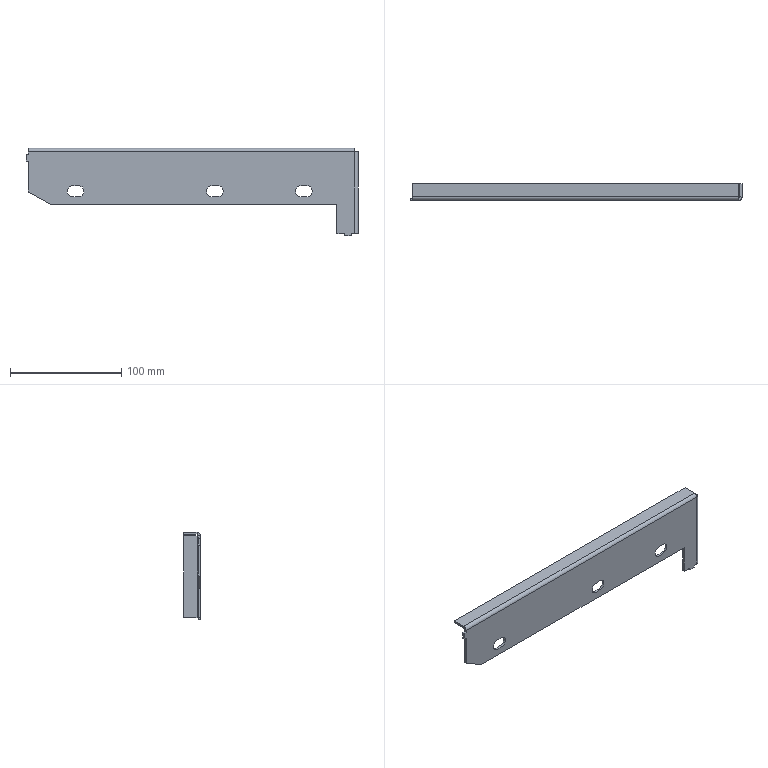Part | SolidWorks | features ICE 3, Cut 2, EdgeFlange 2, FlatPattern 1, SMBaseFlange 1, SheetMetal 1 | 1 solid | 45 faces | box 298 x 15 x 78.5 mm | volume 38712 mm3 | plane 35 | cylinder 10 | commonest cylinder face diameters 10 x6 2 x2 6 x2
STEP:
#1=CARTESIAN_POINT('',(-16.,0.,0.));
#2=VERTEX_POINT('',#1);
#3=CARTESIAN_POINT('',(-9.,0.,0.));
#4=VERTEX_POINT('',#3);
#5=CARTESIAN_POINT('',(-293.,0.,0.));
#6=DIRECTION('',(1.,0.,0.));
#7=VECTOR('',#6,1000.);
#8=LINE('',#5,#7);
#9=EDGE_CURVE('',#2,#4,#8,.T.);
#10=ORIENTED_EDGE('',*,*,#9,.T.);
#11=CARTESIAN_POINT('',(-9.,-2.,0.));
#12=VERTEX_POINT('',#11);
#13=CARTESIAN_POINT('',(-9.,0.,0.));
#14=DIRECTION('',(0.,1.,0.));
#15=VECTOR('',#14,1000.);
#16=LINE('',#13,#15);
#17=EDGE_CURVE('',#12,#4,#16,.T.);
#18=ORIENTED_EDGE('',*,*,#17,.F.);
#19=CARTESIAN_POINT('',(-16.,-2.,0.));
#20=VERTEX_POINT('',#19);
#21=CARTESIAN_POINT('',(-293.,-2.,0.));
#22=DIRECTION('',(1.,0.,0.));
#23=VECTOR('',#22,1000.);
#24=LINE('',#21,#23);
#25=EDGE_CURVE('',#20,#12,#24,.T.);
#26=ORIENTED_EDGE('',*,*,#25,.F.);
#27=CARTESIAN_POINT('',(-16.,0.,0.));
#28=DIRECTION('',(0.,-1.,0.));
#29=VECTOR('',#28,1000.);
#30=LINE('',#27,#29);
#31=EDGE_CURVE('',#2,#20,#30,.T.);
#32=ORIENTED_EDGE('',*,*,#31,.F.);
#33=EDGE_LOOP('',(#10,#18,#26,#32));
#34=FACE_OUTER_BOUND('',#33,.T.);
#35=CARTESIAN_POINT('',(0.,0.,0.));
#36=DIRECTION('',(0.,0.,-1.));
#37=DIRECTION('',(-1.,0.,0.));
#38=AXIS2_PLACEMENT_3D('',#35,#36,#37);
#39=PLANE('',#38);
#40=ADVANCED_FACE('',(#34),#39,.T.);
#41=CARTESIAN_POINT('',(-3.,-2.,0.));
#42=VERTEX_POINT('',#41);
#43=CARTESIAN_POINT('',(0.,-2.,0.));
#44=VERTEX_POINT('',#43);
#45=CARTESIAN_POINT('',(-293.,-2.,0.));
#46=DIRECTION('',(1.,0.,0.));
#47=VECTOR('',#46,1000.);
#48=LINE('',#45,#47);
#49=EDGE_CURVE('',#42,#44,#48,.T.);
#50=ORIENTED_EDGE('',*,*,#49,.F.);
#51=CARTESIAN_POINT('',(-3.,0.,0.));
#52=VERTEX_POINT('',#51);
#53=CARTESIAN_POINT('',(-3.,0.,0.));
#54=DIRECTION('',(0.,-1.,0.));
#55=VECTOR('',#54,1000.);
#56=LINE('',#53,#55);
#57=EDGE_CURVE('',#52,#42,#56,.T.);
#58=ORIENTED_EDGE('',*,*,#57,.F.);
#59=CARTESIAN_POINT('',(0.,0.,0.));
#60=VERTEX_POINT('',#59);
#61=CARTESIAN_POINT('',(-293.,0.,0.));
#62=DIRECTION('',(1.,0.,0.));
#63=VECTOR('',#62,1000.);
#64=LINE('',#61,#63);
#65=EDGE_CURVE('',#52,#60,#64,.T.);
#66=ORIENTED_EDGE('',*,*,#65,.T.);
#67=CARTESIAN_POINT('',(0.,0.,0.));
#68=DIRECTION('',(0.,-1.,0.));
#69=VECTOR('',#68,1000.);
#70=LINE('',#67,#69);
#71=EDGE_CURVE('',#60,#44,#70,.T.);
#72=ORIENTED_EDGE('',*,*,#71,.T.);
#73=EDGE_LOOP('',(#50,#58,#66,#72));
#74=FACE_OUTER_BOUND('',#73,.T.);
#75=CARTESIAN_POINT('',(0.,0.,0.));
#76=DIRECTION('',(0.,0.,-1.));
#77=DIRECTION('',(-1.,0.,0.));
#78=AXIS2_PLACEMENT_3D('',#75,#76,#77);
#79=PLANE('',#78);
#80=ADVANCED_FACE('',(#74),#79,.T.);
#81=CARTESIAN_POINT('',(-293.,0.,73.5));
#82=VERTEX_POINT('',#81);
#83=CARTESIAN_POINT('',(-293.,0.,71.));
#84=VERTEX_POINT('',#83);
#85=CARTESIAN_POINT('',(-293.,0.,73.5));
#86=DIRECTION('',(0.,0.,-1.));
#87=VECTOR('',#86,1000.);
#88=LINE('',#85,#87);
#89=EDGE_CURVE('',#82,#84,#88,.T.);
#90=ORIENTED_EDGE('',*,*,#89,.T.);
#91=CARTESIAN_POINT('',(-293.,-2.,71.));
#92=VERTEX_POINT('',#91);
#93=CARTESIAN_POINT('',(-293.,-2.,71.));
#94=DIRECTION('',(0.,1.,0.));
#95=VECTOR('',#94,1000.);
#96=LINE('',#93,#95);
#97=EDGE_CURVE('',#92,#84,#96,.T.);
#98=ORIENTED_EDGE('',*,*,#97,.F.);
#99=CARTESIAN_POINT('',(-293.,-2.,73.5));
#100=VERTEX_POINT('',#99);
#101=CARTESIAN_POINT('',(-293.,-2.,73.5));
#102=DIRECTION('',(0.,0.,-1.));
#103=VECTOR('',#102,1000.);
#104=LINE('',#101,#103);
#105=EDGE_CURVE('',#100,#92,#104,.T.);
#106=ORIENTED_EDGE('',*,*,#105,.F.);
#107=CARTESIAN_POINT('',(-293.,-2.,73.5));
#108=DIRECTION('',(0.,1.,0.));
#109=VECTOR('',#108,1000.);
#110=LINE('',#107,#109);
#111=EDGE_CURVE('',#100,#82,#110,.T.);
#112=ORIENTED_EDGE('',*,*,#111,.T.);
#113=EDGE_LOOP('',(#90,#98,#106,#112));
#114=FACE_OUTER_BOUND('',#113,.T.);
#115=CARTESIAN_POINT('',(-293.,-2.,73.5));
#116=DIRECTION('',(-1.,0.,0.));
#117=DIRECTION('',(0.,0.,1.));
#118=AXIS2_PLACEMENT_3D('',#115,#116,#117);
#119=PLANE('',#118);
#120=ADVANCED_FACE('',(#114),#119,.T.);
#121=CARTESIAN_POINT('',(-293.,-2.,65.));
#122=VERTEX_POINT('',#121);
#123=CARTESIAN_POINT('',(-293.,-2.,37.2));
#124=VERTEX_POINT('',#123);
#125=CARTESIAN_POINT('',(-293.,-2.,73.5));
#126=DIRECTION('',(0.,0.,-1.));
#127=VECTOR('',#126,1000.);
#128=LINE('',#125,#127);
#129=EDGE_CURVE('',#122,#124,#128,.T.);
#130=ORIENTED_EDGE('',*,*,#129,.F.);
#131=CARTESIAN_POINT('',(-293.,0.,65.));
#132=VERTEX_POINT('',#131);
#133=CARTESIAN_POINT('',(-293.,-2.,65.));
#134=DIRECTION('',(0.,-1.,0.));
#135=VECTOR('',#134,1000.);
#136=LINE('',#133,#135);
#137=EDGE_CURVE('',#132,#122,#136,.T.);
#138=ORIENTED_EDGE('',*,*,#137,.F.);
#139=CARTESIAN_POINT('',(-293.,0.,37.2));
#140=VERTEX_POINT('',#139);
#141=CARTESIAN_POINT('',(-293.,0.,73.5));
#142=DIRECTION('',(0.,0.,-1.));
#143=VECTOR('',#142,1000.);
#144=LINE('',#141,#143);
#145=EDGE_CURVE('',#132,#140,#144,.T.);
#146=ORIENTED_EDGE('',*,*,#145,.T.);
#147=CARTESIAN_POINT('',(-293.,8.,37.2));
#148=DIRECTION('',(0.,-1.,0.));
#149=VECTOR('',#148,1000.);
#150=LINE('',#147,#149);
#151=EDGE_CURVE('',#140,#124,#150,.T.);
#152=ORIENTED_EDGE('',*,*,#151,.T.);
#153=EDGE_LOOP('',(#130,#138,#146,#152));
#154=FACE_OUTER_BOUND('',#153,.T.);
#155=CARTESIAN_POINT('',(-293.,-2.,73.5));
#156=DIRECTION('',(-1.,0.,0.));
#157=DIRECTION('',(0.,0.,1.));
#158=AXIS2_PLACEMENT_3D('',#155,#156,#157);
#159=PLANE('',#158);
#160=ADVANCED_FACE('',(#154),#159,.T.);
#161=CARTESIAN_POINT('',(-253.,-2.,33.));
#162=VERTEX_POINT('',#161);
#163=CARTESIAN_POINT('',(-248.,-2.,33.));
#164=VERTEX_POINT('',#163);
#165=CARTESIAN_POINT('',(-253.,-2.,33.));
#166=DIRECTION('',(1.,0.,0.));
#167=VECTOR('',#166,1000.);
#168=LINE('',#165,#167);
#169=EDGE_CURVE('',#162,#164,#168,.T.);
#170=ORIENTED_EDGE('',*,*,#169,.F.);
#171=CARTESIAN_POINT('',(-253.,-2.,43.));
#172=VERTEX_POINT('',#171);
#173=CARTESIAN_POINT('',(-253.,-2.,38.));
#174=DIRECTION('',(0.,-1.,0.));
#175=DIRECTION('',(0.,0.,-1.));
#176=AXIS2_PLACEMENT_3D('',#173,#174,#175);
#177=CIRCLE('',#176,5.);
#178=EDGE_CURVE('',#172,#162,#177,.T.);
#179=ORIENTED_EDGE('',*,*,#178,.F.);
#180=CARTESIAN_POINT('',(-248.,-2.,43.));
#181=VERTEX_POINT('',#180);
#182=CARTESIAN_POINT('',(-253.,-2.,43.));
#183=DIRECTION('',(-1.,0.,0.));
#184=VECTOR('',#183,1000.);
#185=LINE('',#182,#184);
#186=EDGE_CURVE('',#181,#172,#185,.T.);
#187=ORIENTED_EDGE('',*,*,#186,.F.);
#188=CARTESIAN_POINT('',(-248.,-2.,38.));
#189=DIRECTION('',(0.,-1.,0.));
#190=DIRECTION('',(0.,0.,-1.));
#191=AXIS2_PLACEMENT_3D('',#188,#189,#190);
#192=CIRCLE('',#191,5.);
#193=EDGE_CURVE('',#164,#181,#192,.T.);
#194=ORIENTED_EDGE('',*,*,#193,.F.);
#195=EDGE_LOOP('',(#170,#179,#187,#194));
#196=FACE_BOUND('',#195,.T.);
#197=CARTESIAN_POINT('',(-128.,-2.,33.));
#198=VERTEX_POINT('',#197);
#199=CARTESIAN_POINT('',(-123.,-2.,33.));
#200=VERTEX_POINT('',#199);
#201=CARTESIAN_POINT('',(-128.,-2.,33.));
#202=DIRECTION('',(1.,0.,0.));
#203=VECTOR('',#202,1000.);
#204=LINE('',#201,#203);
#205=EDGE_CURVE('',#198,#200,#204,.T.);
#206=ORIENTED_EDGE('',*,*,#205,.F.);
#207=CARTESIAN_POINT('',(-128.,-2.,43.));
#208=VERTEX_POINT('',#207);
#209=CARTESIAN_POINT('',(-128.,-2.,38.));
#210=DIRECTION('',(0.,-1.,0.));
#211=DIRECTION('',(0.,0.,-1.));
#212=AXIS2_PLACEMENT_3D('',#209,#210,#211);
#213=CIRCLE('',#212,5.);
#214=EDGE_CURVE('',#208,#198,#213,.T.);
#215=ORIENTED_EDGE('',*,*,#214,.F.);
#216=CARTESIAN_POINT('',(-123.,-2.,43.));
#217=VERTEX_POINT('',#216);
#218=CARTESIAN_POINT('',(-128.,-2.,43.));
#219=DIRECTION('',(-1.,0.,0.));
#220=VECTOR('',#219,1000.);
#221=LINE('',#218,#220);
#222=EDGE_CURVE('',#217,#208,#221,.T.);
#223=ORIENTED_EDGE('',*,*,#222,.F.);
#224=CARTESIAN_POINT('',(-123.,-2.,38.));
#225=DIRECTION('',(0.,-1.,0.));
#226=DIRECTION('',(0.,0.,-1.));
#227=AXIS2_PLACEMENT_3D('',#224,#225,#226);
#228=CIRCLE('',#227,5.);
#229=EDGE_CURVE('',#200,#217,#228,.T.);
#230=ORIENTED_EDGE('',*,*,#229,.F.);
#231=EDGE_LOOP('',(#206,#215,#223,#230));
#232=FACE_BOUND('',#231,.T.);
#233=CARTESIAN_POINT('',(-48.,-2.,33.));
#234=VERTEX_POINT('',#233);
#235=CARTESIAN_POINT('',(-43.,-2.,33.));
#236=VERTEX_POINT('',#235);
#237=CARTESIAN_POINT('',(-48.,-2.,33.));
#238=DIRECTION('',(1.,0.,0.));
#239=VECTOR('',#238,1000.);
#240=LINE('',#237,#239);
#241=EDGE_CURVE('',#234,#236,#240,.T.);
#242=ORIENTED_EDGE('',*,*,#241,.F.);
#243=CARTESIAN_POINT('',(-48.,-2.,43.));
#244=VERTEX_POINT('',#243);
#245=CARTESIAN_POINT('',(-48.,-2.,38.));
#246=DIRECTION('',(0.,-1.,0.));
#247=DIRECTION('',(0.,0.,-1.));
#248=AXIS2_PLACEMENT_3D('',#245,#246,#247);
#249=CIRCLE('',#248,5.);
#250=EDGE_CURVE('',#244,#234,#249,.T.);
#251=ORIENTED_EDGE('',*,*,#250,.F.);
#252=CARTESIAN_POINT('',(-43.,-2.,43.));
#253=VERTEX_POINT('',#252);
#254=CARTESIAN_POINT('',(-48.,-2.,43.));
#255=DIRECTION('',(-1.,0.,0.));
#256=VECTOR('',#255,1000.);
#257=LINE('',#254,#256);
#258=EDGE_CURVE('',#253,#244,#257,.T.);
#259=ORIENTED_EDGE('',*,*,#258,.F.);
#260=CARTESIAN_POINT('',(-43.,-2.,38.));
#261=DIRECTION('',(0.,-1.,0.));
#262=DIRECTION('',(0.,0.,-1.));
#263=AXIS2_PLACEMENT_3D('',#260,#261,#262);
#264=CIRCLE('',#263,5.);
#265=EDGE_CURVE('',#236,#253,#264,.T.);
#266=ORIENTED_EDGE('',*,*,#265,.F.);
#267=EDGE_LOOP('',(#242,#251,#259,#266));
#268=FACE_BOUND('',#267,.T.);
#269=ORIENTED_EDGE('',*,*,#105,.T.);
#270=CARTESIAN_POINT('',(-295.,-2.,71.));
#271=VERTEX_POINT('',#270);
#272=CARTESIAN_POINT('',(-295.,-2.,71.));
#273=DIRECTION('',(1.,0.,0.));
#274=VECTOR('',#273,1000.);
#275=LINE('',#272,#274);
#276=EDGE_CURVE('',#271,#92,#275,.T.);
#277=ORIENTED_EDGE('',*,*,#276,.F.);
#278=CARTESIAN_POINT('',(-295.,-2.,65.));
#279=VERTEX_POINT('',#278);
#280=CARTESIAN_POINT('',(-295.,-2.,71.));
#281=DIRECTION('',(0.,0.,1.));
#282=VECTOR('',#281,1000.);
#283=LINE('',#280,#282);
#284=EDGE_CURVE('',#279,#271,#283,.T.);
#285=ORIENTED_EDGE('',*,*,#284,.F.);
#286=CARTESIAN_POINT('',(-295.,-2.,65.));
#287=DIRECTION('',(1.,0.,0.));
#288=VECTOR('',#287,1000.);
#289=LINE('',#286,#288);
#290=EDGE_CURVE('',#279,#122,#289,.T.);
#291=ORIENTED_EDGE('',*,*,#290,.T.);
#292=ORIENTED_EDGE('',*,*,#129,.T.);
#293=CARTESIAN_POINT('',(-273.,-2.,26.2));
#294=VERTEX_POINT('',#293);
#295=CARTESIAN_POINT('',(-293.,-2.,37.2));
#296=DIRECTION('',(-0.8762,0.,0.4819));
#297=VECTOR('',#296,1000.);
#298=LINE('',#295,#297);
#299=EDGE_CURVE('',#294,#124,#298,.T.);
#300=ORIENTED_EDGE('',*,*,#299,.F.);
#301=CARTESIAN_POINT('',(-16.,-2.,26.2));
#302=VERTEX_POINT('',#301);
#303=CARTESIAN_POINT('',(-293.,-2.,26.2));
#304=DIRECTION('',(-1.,0.,0.));
#305=VECTOR('',#304,1000.);
#306=LINE('',#303,#305);
#307=EDGE_CURVE('',#302,#294,#306,.T.);
#308=ORIENTED_EDGE('',*,*,#307,.F.);
#309=CARTESIAN_POINT('',(-16.,-2.,0.));
#310=DIRECTION('',(0.,0.,1.));
#311=VECTOR('',#310,1000.);
#312=LINE('',#309,#311);
#313=EDGE_CURVE('',#20,#302,#312,.T.);
#314=ORIENTED_EDGE('',*,*,#313,.F.);
#315=ORIENTED_EDGE('',*,*,#25,.T.);
#316=CARTESIAN_POINT('',(-9.,-2.,-2.));
#317=VERTEX_POINT('',#316);
#318=CARTESIAN_POINT('',(-9.,-2.,-2.));
#319=DIRECTION('',(0.,0.,1.));
#320=VECTOR('',#319,1000.);
#321=LINE('',#318,#320);
#322=EDGE_CURVE('',#317,#12,#321,.T.);
#323=ORIENTED_EDGE('',*,*,#322,.F.);
#324=CARTESIAN_POINT('',(-3.,-2.,-2.));
#325=VERTEX_POINT('',#324);
#326=CARTESIAN_POINT('',(-9.,-2.,-2.));
#327=DIRECTION('',(-1.,0.,0.));
#328=VECTOR('',#327,1000.);
#329=LINE('',#326,#328);
#330=EDGE_CURVE('',#325,#317,#329,.T.);
#331=ORIENTED_EDGE('',*,*,#330,.F.);
#332=CARTESIAN_POINT('',(-3.,-2.,-2.));
#333=DIRECTION('',(0.,0.,1.));
#334=VECTOR('',#333,1000.);
#335=LINE('',#332,#334);
#336=EDGE_CURVE('',#325,#42,#335,.T.);
#337=ORIENTED_EDGE('',*,*,#336,.T.);
#338=ORIENTED_EDGE('',*,*,#49,.T.);
#339=CARTESIAN_POINT('',(0.,-2.,73.5));
#340=VERTEX_POINT('',#339);
#341=CARTESIAN_POINT('',(0.,-2.,73.5));
#342=DIRECTION('',(0.,0.,-1.));
#343=VECTOR('',#342,1000.);
#344=LINE('',#341,#343);
#345=EDGE_CURVE('',#340,#44,#344,.T.);
#346=ORIENTED_EDGE('',*,*,#345,.F.);
#347=CARTESIAN_POINT('',(-293.,-2.,73.5));
#348=DIRECTION('',(1.,0.,0.));
#349=VECTOR('',#348,1000.);
#350=LINE('',#347,#349);
#351=EDGE_CURVE('',#100,#340,#350,.T.);
#352=ORIENTED_EDGE('',*,*,#351,.F.);
#353=EDGE_LOOP('',(#269,#277,#285,#291,#292,#300,#308,#314,#315,#323,#331,#337,#338,#346,#352));
#354=FACE_OUTER_BOUND('',#353,.T.);
#355=CARTESIAN_POINT('',(-293.,-2.,73.5));
#356=DIRECTION('',(0.,1.,0.));
#357=DIRECTION('',(0.,0.,1.));
#358=AXIS2_PLACEMENT_3D('',#355,#356,#357);
#359=PLANE('',#358);
#360=ADVANCED_FACE('',(#196,#232,#268,#354),#359,.F.);
#361=CARTESIAN_POINT('',(-273.,0.,26.2));
#362=VERTEX_POINT('',#361);
#363=CARTESIAN_POINT('',(-308.328,0.,45.631));
#364=DIRECTION('',(0.8762,0.,-0.4819));
#365=VECTOR('',#364,1000.);
#366=LINE('',#363,#365);
#367=EDGE_CURVE('',#140,#362,#366,.T.);
#368=ORIENTED_EDGE('',*,*,#367,.F.);
#369=ORIENTED_EDGE('',*,*,#145,.F.);
#370=CARTESIAN_POINT('',(-295.,0.,65.));
#371=VERTEX_POINT('',#370);
#372=CARTESIAN_POINT('',(-295.,0.,65.));
#373=DIRECTION('',(1.,0.,0.));
#374=VECTOR('',#373,1000.);
#375=LINE('',#372,#374);
#376=EDGE_CURVE('',#371,#132,#375,.T.);
#377=ORIENTED_EDGE('',*,*,#376,.F.);
#378=CARTESIAN_POINT('',(-295.,0.,71.));
#379=VERTEX_POINT('',#378);
#380=CARTESIAN_POINT('',(-295.,0.,71.));
#381=DIRECTION('',(0.,0.,-1.));
#382=VECTOR('',#381,1000.);
#383=LINE('',#380,#382);
#384=EDGE_CURVE('',#379,#371,#383,.T.);
#385=ORIENTED_EDGE('',*,*,#384,.F.);
#386=CARTESIAN_POINT('',(-295.,0.,71.));
#387=DIRECTION('',(1.,0.,0.));
#388=VECTOR('',#387,1000.);
#389=LINE('',#386,#388);
#390=EDGE_CURVE('',#379,#84,#389,.T.);
#391=ORIENTED_EDGE('',*,*,#390,.T.);
#392=ORIENTED_EDGE('',*,*,#89,.F.);
#393=CARTESIAN_POINT('',(0.,0.,73.5));
#394=VERTEX_POINT('',#393);
#395=CARTESIAN_POINT('',(-293.,0.,73.5));
#396=DIRECTION('',(1.,0.,0.));
#397=VECTOR('',#396,1000.);
#398=LINE('',#395,#397);
#399=EDGE_CURVE('',#82,#394,#398,.T.);
#400=ORIENTED_EDGE('',*,*,#399,.T.);
#401=CARTESIAN_POINT('',(0.,0.,73.5));
#402=DIRECTION('',(0.,0.,-1.));
#403=VECTOR('',#402,1000.);
#404=LINE('',#401,#403);
#405=EDGE_CURVE('',#394,#60,#404,.T.);
#406=ORIENTED_EDGE('',*,*,#405,.T.);
#407=ORIENTED_EDGE('',*,*,#65,.F.);
#408=CARTESIAN_POINT('',(-3.,0.,-2.));
#409=VERTEX_POINT('',#408);
#410=CARTESIAN_POINT('',(-3.,0.,-2.));
#411=DIRECTION('',(0.,0.,1.));
#412=VECTOR('',#411,1000.);
#413=LINE('',#410,#412);
#414=EDGE_CURVE('',#409,#52,#413,.T.);
#415=ORIENTED_EDGE('',*,*,#414,.F.);
#416=CARTESIAN_POINT('',(-9.,0.,-2.));
#417=VERTEX_POINT('',#416);
#418=CARTESIAN_POINT('',(-9.,0.,-2.));
#419=DIRECTION('',(1.,0.,0.));
#420=VECTOR('',#419,1000.);
#421=LINE('',#418,#420);
#422=EDGE_CURVE('',#417,#409,#421,.T.);
#423=ORIENTED_EDGE('',*,*,#422,.F.);
#424=CARTESIAN_POINT('',(-9.,0.,-2.));
#425=DIRECTION('',(0.,0.,1.));
#426=VECTOR('',#425,1000.);
#427=LINE('',#424,#426);
#428=EDGE_CURVE('',#417,#4,#427,.T.);
#429=ORIENTED_EDGE('',*,*,#428,.T.);
#430=ORIENTED_EDGE('',*,*,#9,.F.);
#431=CARTESIAN_POINT('',(-16.,0.,26.2));
#432=VERTEX_POINT('',#431);
#433=CARTESIAN_POINT('',(-16.,0.,73.5));
#434=DIRECTION('',(0.,0.,-1.));
#435=VECTOR('',#434,1000.);
#436=LINE('',#433,#435);
#437=EDGE_CURVE('',#432,#2,#436,.T.);
#438=ORIENTED_EDGE('',*,*,#437,.F.);
#439=CARTESIAN_POINT('',(-293.,0.,26.2));
#440=DIRECTION('',(1.,0.,0.));
#441=VECTOR('',#440,1000.);
#442=LINE('',#439,#441);
#443=EDGE_CURVE('',#362,#432,#442,.T.);
#444=ORIENTED_EDGE('',*,*,#443,.F.);
#445=EDGE_LOOP('',(#368,#369,#377,#385,#391,#392,#400,#406,#407,#415,#423,#429,#430,#438,#444));
#446=FACE_OUTER_BOUND('',#445,.T.);
#447=CARTESIAN_POINT('',(-253.,0.,33.));
#448=VERTEX_POINT('',#447);
#449=CARTESIAN_POINT('',(-253.,0.,43.));
#450=VERTEX_POINT('',#449);
#451=CARTESIAN_POINT('',(-253.,0.,38.));
#452=DIRECTION('',(0.,1.,0.));
#453=DIRECTION('',(0.,0.,1.));
#454=AXIS2_PLACEMENT_3D('',#451,#452,#453);
#455=CIRCLE('',#454,5.);
#456=EDGE_CURVE('',#448,#450,#455,.T.);
#457=ORIENTED_EDGE('',*,*,#456,.F.);
#458=CARTESIAN_POINT('',(-248.,0.,33.));
#459=VERTEX_POINT('',#458);
#460=CARTESIAN_POINT('',(-293.,0.,33.));
#461=DIRECTION('',(-1.,0.,0.));
#462=VECTOR('',#461,1000.);
#463=LINE('',#460,#462);
#464=EDGE_CURVE('',#459,#448,#463,.T.);
#465=ORIENTED_EDGE('',*,*,#464,.F.);
#466=CARTESIAN_POINT('',(-248.,0.,43.));
#467=VERTEX_POINT('',#466);
#468=CARTESIAN_POINT('',(-248.,0.,38.));
#469=DIRECTION('',(0.,1.,0.));
#470=DIRECTION('',(0.,0.,1.));
#471=AXIS2_PLACEMENT_3D('',#468,#469,#470);
#472=CIRCLE('',#471,5.);
#473=EDGE_CURVE('',#467,#459,#472,.T.);
#474=ORIENTED_EDGE('',*,*,#473,.F.);
#475=CARTESIAN_POINT('',(-293.,0.,43.));
#476=DIRECTION('',(1.,0.,0.));
#477=VECTOR('',#476,1000.);
#478=LINE('',#475,#477);
#479=EDGE_CURVE('',#450,#467,#478,.T.);
#480=ORIENTED_EDGE('',*,*,#479,.F.);
#481=EDGE_LOOP('',(#457,#465,#474,#480));
#482=FACE_BOUND('',#481,.T.);
#483=CARTESIAN_POINT('',(-128.,0.,33.));
#484=VERTEX_POINT('',#483);
#485=CARTESIAN_POINT('',(-128.,0.,43.));
#486=VERTEX_POINT('',#485);
#487=CARTESIAN_POINT('',(-128.,0.,38.));
#488=DIRECTION('',(0.,1.,0.));
#489=DIRECTION('',(0.,0.,1.));
#490=AXIS2_PLACEMENT_3D('',#487,#488,#489);
#491=CIRCLE('',#490,5.);
#492=EDGE_CURVE('',#484,#486,#491,.T.);
#493=ORIENTED_EDGE('',*,*,#492,.F.);
#494=CARTESIAN_POINT('',(-123.,0.,33.));
#495=VERTEX_POINT('',#494);
#496=CARTESIAN_POINT('',(-293.,0.,33.));
#497=DIRECTION('',(-1.,0.,0.));
#498=VECTOR('',#497,1000.);
#499=LINE('',#496,#498);
#500=EDGE_CURVE('',#495,#484,#499,.T.);
#501=ORIENTED_EDGE('',*,*,#500,.F.);
#502=CARTESIAN_POINT('',(-123.,0.,43.));
#503=VERTEX_POINT('',#502);
#504=CARTESIAN_POINT('',(-123.,0.,38.));
#505=DIRECTION('',(0.,1.,0.));
#506=DIRECTION('',(0.,0.,1.));
#507=AXIS2_PLACEMENT_3D('',#504,#505,#506);
#508=CIRCLE('',#507,5.);
#509=EDGE_CURVE('',#503,#495,#508,.T.);
#510=ORIENTED_EDGE('',*,*,#509,.F.);
#511=CARTESIAN_POINT('',(-293.,0.,43.));
#512=DIRECTION('',(1.,0.,0.));
#513=VECTOR('',#512,1000.);
#514=LINE('',#511,#513);
#515=EDGE_CURVE('',#486,#503,#514,.T.);
#516=ORIENTED_EDGE('',*,*,#515,.F.);
#517=EDGE_LOOP('',(#493,#501,#510,#516));
#518=FACE_BOUND('',#517,.T.);
#519=CARTESIAN_POINT('',(-48.,0.,33.));
#520=VERTEX_POINT('',#519);
#521=CARTESIAN_POINT('',(-48.,0.,43.));
#522=VERTEX_POINT('',#521);
#523=CARTESIAN_POINT('',(-48.,0.,38.));
#524=DIRECTION('',(0.,1.,0.));
#525=DIRECTION('',(0.,0.,1.));
#526=AXIS2_PLACEMENT_3D('',#523,#524,#525);
#527=CIRCLE('',#526,5.);
#528=EDGE_CURVE('',#520,#522,#527,.T.);
#529=ORIENTED_EDGE('',*,*,#528,.F.);
#530=CARTESIAN_POINT('',(-43.,0.,33.));
#531=VERTEX_POINT('',#530);
#532=CARTESIAN_POINT('',(-293.,0.,33.));
#533=DIRECTION('',(-1.,0.,0.));
#534=VECTOR('',#533,1000.);
#535=LINE('',#532,#534);
#536=EDGE_CURVE('',#531,#520,#535,.T.);
#537=ORIENTED_EDGE('',*,*,#536,.F.);
#538=CARTESIAN_POINT('',(-43.,0.,43.));
#539=VERTEX_POINT('',#538);
#540=CARTESIAN_POINT('',(-43.,0.,38.));
#541=DIRECTION('',(0.,1.,0.));
#542=DIRECTION('',(0.,0.,1.));
#543=AXIS2_PLACEMENT_3D('',#540,#541,#542);
#544=CIRCLE('',#543,5.);
#545=EDGE_CURVE('',#539,#531,#544,.T.);
#546=ORIENTED_EDGE('',*,*,#545,.F.);
#547=CARTESIAN_POINT('',(-293.,0.,43.));
#548=DIRECTION('',(1.,0.,0.));
#549=VECTOR('',#548,1000.);
#550=LINE('',#547,#549);
#551=EDGE_CURVE('',#522,#539,#550,.T.);
#552=ORIENTED_EDGE('',*,*,#551,.F.);
#553=EDGE_LOOP('',(#529,#537,#546,#552));
#554=FACE_BOUND('',#553,.T.);
#555=CARTESIAN_POINT('',(-293.,0.,73.5));
#556=DIRECTION('',(0.,1.,0.));
#557=DIRECTION('',(0.,0.,1.));
#558=AXIS2_PLACEMENT_3D('',#555,#556,#557);
#559=PLANE('',#558);
#560=ADVANCED_FACE('',(#446,#482,#518,#554),#559,.T.);
#561=CARTESIAN_POINT('',(-293.,1.,74.5));
#562=VERTEX_POINT('',#561);
#563=CARTESIAN_POINT('',(-293.,1.,76.5));
#564=VERTEX_POINT('',#563);
#565=CARTESIAN_POINT('',(-293.,1.,76.5));
#566=DIRECTION('',(0.,0.,1.));
#567=VECTOR('',#566,1000.);
#568=LINE('',#565,#567);
#569=EDGE_CURVE('',#562,#564,#568,.T.);
#570=ORIENTED_EDGE('',*,*,#569,.F.);
#571=CARTESIAN_POINT('',(-293.,1.,73.5));
#572=DIRECTION('',(-1.,0.,0.));
#573=DIRECTION('',(0.,0.,-1.));
#574=AXIS2_PLACEMENT_3D('',#571,#572,#573);
#575=CIRCLE('',#574,1.);
#576=EDGE_CURVE('',#82,#562,#575,.T.);
#577=ORIENTED_EDGE('',*,*,#576,.F.);
#578=ORIENTED_EDGE('',*,*,#111,.F.);
#579=CARTESIAN_POINT('',(-293.,1.,73.5));
#580=DIRECTION('',(-1.,0.,0.));
#581=DIRECTION('',(0.,0.,-1.));
#582=AXIS2_PLACEMENT_3D('',#579,#580,#581);
#583=CIRCLE('',#582,3.);
#584=EDGE_CURVE('',#100,#564,#583,.T.);
#585=ORIENTED_EDGE('',*,*,#584,.T.);
#586=EDGE_LOOP('',(#570,#577,#578,#585));
#587=FACE_OUTER_BOUND('',#586,.T.);
#588=CARTESIAN_POINT('',(-293.,1.,73.5));
#589=DIRECTION('',(-1.,0.,0.));
#590=DIRECTION('',(0.,0.,1.));
#591=AXIS2_PLACEMENT_3D('',#588,#589,#590);
#592=PLANE('',#591);
#593=ADVANCED_FACE('',(#587),#592,.T.);
#594=CARTESIAN_POINT('',(0.,1.,74.5));
#595=VERTEX_POINT('',#594);
#596=CARTESIAN_POINT('',(0.,1.,73.5));
#597=DIRECTION('',(1.,0.,0.));
#598=DIRECTION('',(0.,0.,-1.));
#599=AXIS2_PLACEMENT_3D('',#596,#597,#598);
#600=CIRCLE('',#599,1.);
#601=EDGE_CURVE('',#595,#394,#600,.T.);
#602=ORIENTED_EDGE('',*,*,#601,.F.);
#603=CARTESIAN_POINT('',(0.,1.,76.5));
#604=VERTEX_POINT('',#603);
#605=CARTESIAN_POINT('',(0.,1.,74.5));
#606=DIRECTION('',(0.,0.,1.));
#607=VECTOR('',#606,1000.);
#608=LINE('',#605,#607);
#609=EDGE_CURVE('',#595,#604,#608,.T.);
#610=ORIENTED_EDGE('',*,*,#609,.T.);
#611=CARTESIAN_POINT('',(0.,1.,73.5));
#612=DIRECTION('',(1.,0.,0.));
#613=DIRECTION('',(0.,0.,-1.));
#614=AXIS2_PLACEMENT_3D('',#611,#612,#613);
#615=CIRCLE('',#614,3.);
#616=EDGE_CURVE('',#604,#340,#615,.T.);
#617=ORIENTED_EDGE('',*,*,#616,.T.);
#618=CARTESIAN_POINT('',(0.,0.,73.5));
#619=DIRECTION('',(0.,-1.,0.));
#620=VECTOR('',#619,1000.);
#621=LINE('',#618,#620);
#622=EDGE_CURVE('',#394,#340,#621,.T.);
#623=ORIENTED_EDGE('',*,*,#622,.F.);
#624=EDGE_LOOP('',(#602,#610,#617,#623));
#625=FACE_OUTER_BOUND('',#624,.T.);
#626=CARTESIAN_POINT('',(0.,1.,73.5));
#627=DIRECTION('',(-1.,0.,0.));
#628=DIRECTION('',(0.,0.,1.));
#629=AXIS2_PLACEMENT_3D('',#626,#627,#628);
#630=PLANE('',#629);
#631=ADVANCED_FACE('',(#625),#630,.F.);
#632=ORIENTED_EDGE('',*,*,#351,.T.);
#633=ORIENTED_EDGE('',*,*,#616,.F.);
#634=CARTESIAN_POINT('',(-293.,1.,76.5));
#635=DIRECTION('',(-1.,0.,0.));
#636=VECTOR('',#635,1000.);
#637=LINE('',#634,#636);
#638=EDGE_CURVE('',#604,#564,#637,.T.);
#639=ORIENTED_EDGE('',*,*,#638,.T.);
#640=ORIENTED_EDGE('',*,*,#584,.F.);
#641=EDGE_LOOP('',(#632,#633,#639,#640));
#642=FACE_OUTER_BOUND('',#641,.T.);
#643=CARTESIAN_POINT('',(0.,1.,73.5));
#644=DIRECTION('',(1.,0.,0.));
#645=DIRECTION('',(0.,0.,1.));
#646=AXIS2_PLACEMENT_3D('',#643,#644,#645);
#647=CYLINDRICAL_SURFACE('',#646,3.);
#648=ADVANCED_FACE('',(#642),#647,.T.);
#649=ORIENTED_EDGE('',*,*,#399,.F.);
#650=ORIENTED_EDGE('',*,*,#576,.T.);
#651=CARTESIAN_POINT('',(-293.,1.,74.5));
#652=DIRECTION('',(1.,0.,0.));
#653=VECTOR('',#652,1000.);
#654=LINE('',#651,#653);
#655=EDGE_CURVE('',#562,#595,#654,.T.);
#656=ORIENTED_EDGE('',*,*,#655,.T.);
#657=ORIENTED_EDGE('',*,*,#601,.T.);
#658=EDGE_LOOP('',(#649,#650,#656,#657));
#659=FACE_OUTER_BOUND('',#658,.T.);
#660=CARTESIAN_POINT('',(0.,1.,73.5));
#661=DIRECTION('',(1.,0.,0.));
#662=DIRECTION('',(0.,0.,1.));
#663=AXIS2_PLACEMENT_3D('',#660,#661,#662);
#664=CYLINDRICAL_SURFACE('',#663,1.);
#665=ADVANCED_FACE('',(#659),#664,.F.);
#666=ORIENTED_EDGE('',*,*,#569,.T.);
#667=CARTESIAN_POINT('',(-293.,13.,76.5));
#668=VERTEX_POINT('',#667);
#669=CARTESIAN_POINT('',(-293.,0.,76.5));
#670=DIRECTION('',(0.,-1.,0.));
#671=VECTOR('',#670,1000.);
#672=LINE('',#669,#671);
#673=EDGE_CURVE('',#668,#564,#672,.T.);
#674=ORIENTED_EDGE('',*,*,#673,.F.);
#675=CARTESIAN_POINT('',(-293.,13.,74.5));
#676=VERTEX_POINT('',#675);
#677=CARTESIAN_POINT('',(-293.,13.,76.5));
#678=DIRECTION('',(0.,0.,-1.));
#679=VECTOR('',#678,1000.);
#680=LINE('',#677,#679);
#681=EDGE_CURVE('',#668,#676,#680,.T.);
#682=ORIENTED_EDGE('',*,*,#681,.T.);
#683=CARTESIAN_POINT('',(-293.,0.,74.5));
#684=DIRECTION('',(0.,-1.,0.));
#685=VECTOR('',#684,1000.);
#686=LINE('',#683,#685);
#687=EDGE_CURVE('',#676,#562,#686,.T.);
#688=ORIENTED_EDGE('',*,*,#687,.T.);
#689=EDGE_LOOP('',(#666,#674,#682,#688));
#690=FACE_OUTER_BOUND('',#689,.T.);
#691=CARTESIAN_POINT('',(-293.,0.,76.5));
#692=DIRECTION('',(1.,0.,0.));
#693=DIRECTION('',(0.,0.,-1.));
#694=AXIS2_PLACEMENT_3D('',#691,#692,#693);
#695=PLANE('',#694);
#696=ADVANCED_FACE('',(#690),#695,.F.);
#697=ORIENTED_EDGE('',*,*,#609,.F.);
#698=CARTESIAN_POINT('',(0.,13.,74.5));
#699=VERTEX_POINT('',#698);
#700=CARTESIAN_POINT('',(0.,13.,74.5));
#701=DIRECTION('',(0.,1.,0.));
#702=VECTOR('',#701,1000.);
#703=LINE('',#700,#702);
#704=EDGE_CURVE('',#595,#699,#703,.T.);
#705=ORIENTED_EDGE('',*,*,#704,.T.);
#706=CARTESIAN_POINT('',(0.,13.,76.5));
#707=VERTEX_POINT('',#706);
#708=CARTESIAN_POINT('',(0.,13.,76.5));
#709=DIRECTION('',(0.,0.,-1.));
#710=VECTOR('',#709,1000.);
#711=LINE('',#708,#710);
#712=EDGE_CURVE('',#707,#699,#711,.T.);
#713=ORIENTED_EDGE('',*,*,#712,.F.);
#714=CARTESIAN_POINT('',(0.,0.,76.5));
#715=DIRECTION('',(0.,1.,0.));
#716=VECTOR('',#715,1000.);
#717=LINE('',#714,#716);
#718=EDGE_CURVE('',#604,#707,#717,.T.);
#719=ORIENTED_EDGE('',*,*,#718,.F.);
#720=EDGE_LOOP('',(#697,#705,#713,#719));
#721=FACE_OUTER_BOUND('',#720,.T.);
#722=CARTESIAN_POINT('',(0.,13.,76.5));
#723=DIRECTION('',(-1.,0.,0.));
#724=DIRECTION('',(0.,-1.,0.));
#725=AXIS2_PLACEMENT_3D('',#722,#723,#724);
#726=PLANE('',#725);
#727=ADVANCED_FACE('',(#721),#726,.F.);
#728=ORIENTED_EDGE('',*,*,#638,.F.);
#729=ORIENTED_EDGE('',*,*,#718,.T.);
#730=CARTESIAN_POINT('',(0.,13.,76.5));
#731=DIRECTION('',(-1.,0.,0.));
#732=VECTOR('',#731,1000.);
#733=LINE('',#730,#732);
#734=EDGE_CURVE('',#707,#668,#733,.T.);
#735=ORIENTED_EDGE('',*,*,#734,.T.);
#736=ORIENTED_EDGE('',*,*,#673,.T.);
#737=EDGE_LOOP('',(#728,#729,#735,#736));
#738=FACE_OUTER_BOUND('',#737,.T.);
#739=CARTESIAN_POINT('',(0.,0.,76.5));
#740=DIRECTION('',(0.,0.,-1.));
#741=DIRECTION('',(-1.,0.,0.));
#742=AXIS2_PLACEMENT_3D('',#739,#740,#741);
#743=PLANE('',#742);
#744=ADVANCED_FACE('',(#738),#743,.F.);
#745=ORIENTED_EDGE('',*,*,#704,.F.);
#746=ORIENTED_EDGE('',*,*,#655,.F.);
#747=ORIENTED_EDGE('',*,*,#687,.F.);
#748=CARTESIAN_POINT('',(-293.,13.,74.5));
#749=DIRECTION('',(-1.,0.,0.));
#750=VECTOR('',#749,1000.);
#751=LINE('',#748,#750);
#752=EDGE_CURVE('',#699,#676,#751,.T.);
#753=ORIENTED_EDGE('',*,*,#752,.F.);
#754=EDGE_LOOP('',(#745,#746,#747,#753));
#755=FACE_OUTER_BOUND('',#754,.T.);
#756=CARTESIAN_POINT('',(0.,0.,74.5));
#757=DIRECTION('',(0.,0.,-1.));
#758=DIRECTION('',(-1.,0.,0.));
#759=AXIS2_PLACEMENT_3D('',#756,#757,#758);
#760=PLANE('',#759);
#761=ADVANCED_FACE('',(#755),#760,.T.);
#762=ORIENTED_EDGE('',*,*,#752,.T.);
#763=ORIENTED_EDGE('',*,*,#681,.F.);
#764=ORIENTED_EDGE('',*,*,#734,.F.);
#765=ORIENTED_EDGE('',*,*,#712,.T.);
#766=EDGE_LOOP('',(#762,#763,#764,#765));
#767=FACE_OUTER_BOUND('',#766,.T.);
#768=CARTESIAN_POINT('',(-293.,13.,76.5));
#769=DIRECTION('',(0.,-1.,0.));
#770=DIRECTION('',(0.,0.,-1.));
#771=AXIS2_PLACEMENT_3D('',#768,#769,#770);
#772=PLANE('',#771);
#773=ADVANCED_FACE('',(#767),#772,.F.);
#774=CARTESIAN_POINT('',(1.,1.,73.5));
#775=VERTEX_POINT('',#774);
#776=CARTESIAN_POINT('',(3.,1.,73.5));
#777=VERTEX_POINT('',#776);
#778=CARTESIAN_POINT('',(3.,1.,73.5));
#779=DIRECTION('',(1.,0.,0.));
#780=VECTOR('',#779,1000.);
#781=LINE('',#778,#780);
#782=EDGE_CURVE('',#775,#777,#781,.T.);
#783=ORIENTED_EDGE('',*,*,#782,.F.);
#784=CARTESIAN_POINT('',(0.,1.,73.5));
#785=DIRECTION('',(0.,0.,1.));
#786=DIRECTION('',(-1.,0.,0.));
#787=AXIS2_PLACEMENT_3D('',#784,#785,#786);
#788=CIRCLE('',#787,1.);
#789=EDGE_CURVE('',#394,#775,#788,.T.);
#790=ORIENTED_EDGE('',*,*,#789,.F.);
#791=ORIENTED_EDGE('',*,*,#622,.T.);
#792=CARTESIAN_POINT('',(0.,1.,73.5));
#793=DIRECTION('',(0.,0.,1.));
#794=DIRECTION('',(-1.,0.,0.));
#795=AXIS2_PLACEMENT_3D('',#792,#793,#794);
#796=CIRCLE('',#795,3.);
#797=EDGE_CURVE('',#340,#777,#796,.T.);
#798=ORIENTED_EDGE('',*,*,#797,.T.);
#799=EDGE_LOOP('',(#783,#790,#791,#798));
#800=FACE_OUTER_BOUND('',#799,.T.);
#801=CARTESIAN_POINT('',(0.,1.,73.5));
#802=DIRECTION('',(0.,0.,1.));
#803=DIRECTION('',(1.,0.,0.));
#804=AXIS2_PLACEMENT_3D('',#801,#802,#803);
#805=PLANE('',#804);
#806=ADVANCED_FACE('',(#800),#805,.T.);
#807=CARTESIAN_POINT('',(1.,1.,0.));
#808=VERTEX_POINT('',#807);
#809=CARTESIAN_POINT('',(0.,1.,0.));
#810=DIRECTION('',(0.,0.,-1.));
#811=DIRECTION('',(-1.,0.,0.));
#812=AXIS2_PLACEMENT_3D('',#809,#810,#811);
#813=CIRCLE('',#812,1.);
#814=EDGE_CURVE('',#808,#60,#813,.T.);
#815=ORIENTED_EDGE('',*,*,#814,.F.);
#816=CARTESIAN_POINT('',(3.,1.,0.));
#817=VERTEX_POINT('',#816);
#818=CARTESIAN_POINT('',(1.,1.,0.));
#819=DIRECTION('',(1.,0.,0.));
#820=VECTOR('',#819,1000.);
#821=LINE('',#818,#820);
#822=EDGE_CURVE('',#808,#817,#821,.T.);
#823=ORIENTED_EDGE('',*,*,#822,.T.);
#824=CARTESIAN_POINT('',(0.,1.,0.));
#825=DIRECTION('',(0.,0.,-1.));
#826=DIRECTION('',(-1.,0.,0.));
#827=AXIS2_PLACEMENT_3D('',#824,#825,#826);
#828=CIRCLE('',#827,3.);
#829=EDGE_CURVE('',#817,#44,#828,.T.);
#830=ORIENTED_EDGE('',*,*,#829,.T.);
#831=ORIENTED_EDGE('',*,*,#71,.F.);
#832=EDGE_LOOP('',(#815,#823,#830,#831));
#833=FACE_OUTER_BOUND('',#832,.T.);
#834=CARTESIAN_POINT('',(0.,1.,0.));
#835=DIRECTION('',(0.,0.,1.));
#836=DIRECTION('',(1.,0.,0.));
#837=AXIS2_PLACEMENT_3D('',#834,#835,#836);
#838=PLANE('',#837);
#839=ADVANCED_FACE('',(#833),#838,.F.);
#840=ORIENTED_EDGE('',*,*,#345,.T.);
#841=ORIENTED_EDGE('',*,*,#829,.F.);
#842=CARTESIAN_POINT('',(3.,1.,73.5));
#843=DIRECTION('',(0.,0.,1.));
#844=VECTOR('',#843,1000.);
#845=LINE('',#842,#844);
#846=EDGE_CURVE('',#817,#777,#845,.T.);
#847=ORIENTED_EDGE('',*,*,#846,.T.);
#848=ORIENTED_EDGE('',*,*,#797,.F.);
#849=EDGE_LOOP('',(#840,#841,#847,#848));
#850=FACE_OUTER_BOUND('',#849,.T.);
#851=CARTESIAN_POINT('',(0.,1.,0.));
#852=DIRECTION('',(0.,0.,-1.));
#853=DIRECTION('',(1.,0.,0.));
#854=AXIS2_PLACEMENT_3D('',#851,#852,#853);
#855=CYLINDRICAL_SURFACE('',#854,3.);
#856=ADVANCED_FACE('',(#850),#855,.T.);
#857=ORIENTED_EDGE('',*,*,#405,.F.);
#858=ORIENTED_EDGE('',*,*,#789,.T.);
#859=CARTESIAN_POINT('',(1.,1.,73.5));
#860=DIRECTION('',(0.,0.,-1.));
#861=VECTOR('',#860,1000.);
#862=LINE('',#859,#861);
#863=EDGE_CURVE('',#775,#808,#862,.T.);
#864=ORIENTED_EDGE('',*,*,#863,.T.);
#865=ORIENTED_EDGE('',*,*,#814,.T.);
#866=EDGE_LOOP('',(#857,#858,#864,#865));
#867=FACE_OUTER_BOUND('',#866,.T.);
#868=CARTESIAN_POINT('',(0.,1.,0.));
#869=DIRECTION('',(0.,0.,-1.));
#870=DIRECTION('',(1.,0.,0.));
#871=AXIS2_PLACEMENT_3D('',#868,#869,#870);
#872=CYLINDRICAL_SURFACE('',#871,1.);
#873=ADVANCED_FACE('',(#867),#872,.F.);
#874=ORIENTED_EDGE('',*,*,#782,.T.);
#875=CARTESIAN_POINT('',(3.,13.,73.5));
#876=VERTEX_POINT('',#875);
#877=CARTESIAN_POINT('',(3.,0.,73.5));
#878=DIRECTION('',(0.,-1.,0.));
#879=VECTOR('',#878,1000.);
#880=LINE('',#877,#879);
#881=EDGE_CURVE('',#876,#777,#880,.T.);
#882=ORIENTED_EDGE('',*,*,#881,.F.);
#883=CARTESIAN_POINT('',(1.,13.,73.5));
#884=VERTEX_POINT('',#883);
#885=CARTESIAN_POINT('',(3.,13.,73.5));
#886=DIRECTION('',(-1.,0.,0.));
#887=VECTOR('',#886,1000.);
#888=LINE('',#885,#887);
#889=EDGE_CURVE('',#876,#884,#888,.T.);
#890=ORIENTED_EDGE('',*,*,#889,.T.);
#891=CARTESIAN_POINT('',(1.,0.,73.5));
#892=DIRECTION('',(0.,-1.,0.));
#893=VECTOR('',#892,1000.);
#894=LINE('',#891,#893);
#895=EDGE_CURVE('',#884,#775,#894,.T.);
#896=ORIENTED_EDGE('',*,*,#895,.T.);
#897=EDGE_LOOP('',(#874,#882,#890,#896));
#898=FACE_OUTER_BOUND('',#897,.T.);
#899=CARTESIAN_POINT('',(3.,0.,73.5));
#900=DIRECTION('',(0.,0.,-1.));
#901=DIRECTION('',(-1.,0.,0.));
#902=AXIS2_PLACEMENT_3D('',#899,#900,#901);
#903=PLANE('',#902);
#904=ADVANCED_FACE('',(#898),#903,.F.);
#905=ORIENTED_EDGE('',*,*,#822,.F.);
#906=CARTESIAN_POINT('',(1.,13.,0.));
#907=VERTEX_POINT('',#906);
#908=CARTESIAN_POINT('',(1.,13.,0.));
#909=DIRECTION('',(0.,1.,0.));
#910=VECTOR('',#909,1000.);
#911=LINE('',#908,#910);
#912=EDGE_CURVE('',#808,#907,#911,.T.);
#913=ORIENTED_EDGE('',*,*,#912,.T.);
#914=CARTESIAN_POINT('',(3.,13.,0.));
#915=VERTEX_POINT('',#914);
#916=CARTESIAN_POINT('',(3.,13.,0.));
#917=DIRECTION('',(-1.,0.,0.));
#918=VECTOR('',#917,1000.);
#919=LINE('',#916,#918);
#920=EDGE_CURVE('',#915,#907,#919,.T.);
#921=ORIENTED_EDGE('',*,*,#920,.F.);
#922=CARTESIAN_POINT('',(3.,0.,0.));
#923=DIRECTION('',(0.,1.,0.));
#924=VECTOR('',#923,1000.);
#925=LINE('',#922,#924);
#926=EDGE_CURVE('',#817,#915,#925,.T.);
#927=ORIENTED_EDGE('',*,*,#926,.F.);
#928=EDGE_LOOP('',(#905,#913,#921,#927));
#929=FACE_OUTER_BOUND('',#928,.T.);
#930=CARTESIAN_POINT('',(3.,13.,0.));
#931=DIRECTION('',(0.,0.,1.));
#932=DIRECTION('',(1.,0.,0.));
#933=AXIS2_PLACEMENT_3D('',#930,#931,#932);
#934=PLANE('',#933);
#935=ADVANCED_FACE('',(#929),#934,.F.);
#936=ORIENTED_EDGE('',*,*,#846,.F.);
#937=ORIENTED_EDGE('',*,*,#926,.T.);
#938=CARTESIAN_POINT('',(3.,13.,0.));
#939=DIRECTION('',(0.,0.,1.));
#940=VECTOR('',#939,1000.);
#941=LINE('',#938,#940);
#942=EDGE_CURVE('',#915,#876,#941,.T.);
#943=ORIENTED_EDGE('',*,*,#942,.T.);
#944=ORIENTED_EDGE('',*,*,#881,.T.);
#945=EDGE_LOOP('',(#936,#937,#943,#944));
#946=FACE_OUTER_BOUND('',#945,.T.);
#947=CARTESIAN_POINT('',(3.,0.,0.));
#948=DIRECTION('',(-1.,0.,0.));
#949=DIRECTION('',(0.,-1.,0.));
#950=AXIS2_PLACEMENT_3D('',#947,#948,#949);
#951=PLANE('',#950);
#952=ADVANCED_FACE('',(#946),#951,.F.);
#953=ORIENTED_EDGE('',*,*,#912,.F.);
#954=ORIENTED_EDGE('',*,*,#863,.F.);
#955=ORIENTED_EDGE('',*,*,#895,.F.);
#956=CARTESIAN_POINT('',(1.,13.,73.5));
#957=DIRECTION('',(0.,0.,1.));
#958=VECTOR('',#957,1000.);
#959=LINE('',#956,#958);
#960=EDGE_CURVE('',#907,#884,#959,.T.);
#961=ORIENTED_EDGE('',*,*,#960,.F.);
#962=EDGE_LOOP('',(#953,#954,#955,#961));
#963=FACE_OUTER_BOUND('',#962,.T.);
#964=CARTESIAN_POINT('',(1.,0.,0.));
#965=DIRECTION('',(-1.,0.,0.));
#966=DIRECTION('',(0.,-1.,0.));
#967=AXIS2_PLACEMENT_3D('',#964,#965,#966);
#968=PLANE('',#967);
#969=ADVANCED_FACE('',(#963),#968,.T.);
#970=ORIENTED_EDGE('',*,*,#960,.T.);
#971=ORIENTED_EDGE('',*,*,#889,.F.);
#972=ORIENTED_EDGE('',*,*,#942,.F.);
#973=ORIENTED_EDGE('',*,*,#920,.T.);
#974=EDGE_LOOP('',(#970,#971,#972,#973));
#975=FACE_OUTER_BOUND('',#974,.T.);
#976=CARTESIAN_POINT('',(3.,13.,73.5));
#977=DIRECTION('',(0.,-1.,0.));
#978=DIRECTION('',(1.,0.,0.));
#979=AXIS2_PLACEMENT_3D('',#976,#977,#978);
#980=PLANE('',#979);
#981=ADVANCED_FACE('',(#975),#980,.F.);
#982=ORIENTED_EDGE('',*,*,#307,.T.);
#983=CARTESIAN_POINT('',(-273.,8.,26.2));
#984=DIRECTION('',(0.,1.,0.));
#985=VECTOR('',#984,1000.);
#986=LINE('',#983,#985);
#987=EDGE_CURVE('',#294,#362,#986,.T.);
#988=ORIENTED_EDGE('',*,*,#987,.T.);
#989=ORIENTED_EDGE('',*,*,#443,.T.);
#990=CARTESIAN_POINT('',(-16.,8.,26.2));
#991=DIRECTION('',(0.,-1.,0.));
#992=VECTOR('',#991,1000.);
#993=LINE('',#990,#992);
#994=EDGE_CURVE('',#432,#302,#993,.T.);
#995=ORIENTED_EDGE('',*,*,#994,.T.);
#996=EDGE_LOOP('',(#982,#988,#989,#995));
#997=FACE_OUTER_BOUND('',#996,.T.);
#998=CARTESIAN_POINT('',(-293.,8.,26.2));
#999=DIRECTION('',(0.,0.,1.));
#1000=DIRECTION('',(1.,0.,0.));
#1001=AXIS2_PLACEMENT_3D('',#998,#999,#1000);
#1002=PLANE('',#1001);
#1003=ADVANCED_FACE('',(#997),#1002,.F.);
#1004=ORIENTED_EDGE('',*,*,#437,.T.);
#1005=ORIENTED_EDGE('',*,*,#31,.T.);
#1006=ORIENTED_EDGE('',*,*,#313,.T.);
#1007=ORIENTED_EDGE('',*,*,#994,.F.);
#1008=EDGE_LOOP('',(#1004,#1005,#1006,#1007));
#1009=FACE_OUTER_BOUND('',#1008,.T.);
#1010=CARTESIAN_POINT('',(-16.,8.,0.));
#1011=DIRECTION('',(1.,0.,0.));
#1012=DIRECTION('',(0.,0.,-1.));
#1013=AXIS2_PLACEMENT_3D('',#1010,#1011,#1012);
#1014=PLANE('',#1013);
#1015=ADVANCED_FACE('',(#1009),#1014,.F.);
#1016=ORIENTED_EDGE('',*,*,#528,.T.);
#1017=CARTESIAN_POINT('',(-48.,8.,43.));
#1018=DIRECTION('',(0.,-1.,0.));
#1019=VECTOR('',#1018,1000.);
#1020=LINE('',#1017,#1019);
#1021=EDGE_CURVE('',#522,#244,#1020,.T.);
#1022=ORIENTED_EDGE('',*,*,#1021,.T.);
#1023=ORIENTED_EDGE('',*,*,#250,.T.);
#1024=CARTESIAN_POINT('',(-48.,8.,33.));
#1025=DIRECTION('',(0.,-1.,0.));
#1026=VECTOR('',#1025,1000.);
#1027=LINE('',#1024,#1026);
#1028=EDGE_CURVE('',#520,#234,#1027,.T.);
#1029=ORIENTED_EDGE('',*,*,#1028,.F.);
#1030=EDGE_LOOP('',(#1016,#1022,#1023,#1029));
#1031=FACE_OUTER_BOUND('',#1030,.T.);
#1032=CARTESIAN_POINT('',(-48.,8.,38.));
#1033=DIRECTION('',(0.,-1.,0.));
#1034=DIRECTION('',(0.,0.,-1.));
#1035=AXIS2_PLACEMENT_3D('',#1032,#1033,#1034);
#1036=CYLINDRICAL_SURFACE('',#1035,5.);
#1037=ADVANCED_FACE('',(#1031),#1036,.F.);
#1038=ORIENTED_EDGE('',*,*,#551,.T.);
#1039=CARTESIAN_POINT('',(-43.,8.,43.));
#1040=DIRECTION('',(0.,-1.,0.));
#1041=VECTOR('',#1040,1000.);
#1042=LINE('',#1039,#1041);
#1043=EDGE_CURVE('',#539,#253,#1042,.T.);
#1044=ORIENTED_EDGE('',*,*,#1043,.T.);
#1045=ORIENTED_EDGE('',*,*,#258,.T.);
#1046=ORIENTED_EDGE('',*,*,#1021,.F.);
#1047=EDGE_LOOP('',(#1038,#1044,#1045,#1046));
#1048=FACE_OUTER_BOUND('',#1047,.T.);
#1049=CARTESIAN_POINT('',(-48.,8.,43.));
#1050=DIRECTION('',(0.,0.,1.));
#1051=DIRECTION('',(1.,0.,0.));
#1052=AXIS2_PLACEMENT_3D('',#1049,#1050,#1051);
#1053=PLANE('',#1052);
#1054=ADVANCED_FACE('',(#1048),#1053,.F.);
#1055=ORIENTED_EDGE('',*,*,#545,.T.);
#1056=CARTESIAN_POINT('',(-43.,8.,33.));
#1057=DIRECTION('',(0.,-1.,0.));
#1058=VECTOR('',#1057,1000.);
#1059=LINE('',#1056,#1058);
#1060=EDGE_CURVE('',#531,#236,#1059,.T.);
#1061=ORIENTED_EDGE('',*,*,#1060,.T.);
#1062=ORIENTED_EDGE('',*,*,#265,.T.);
#1063=ORIENTED_EDGE('',*,*,#1043,.F.);
#1064=EDGE_LOOP('',(#1055,#1061,#1062,#1063));
#1065=FACE_OUTER_BOUND('',#1064,.T.);
#1066=CARTESIAN_POINT('',(-43.,8.,38.));
#1067=DIRECTION('',(0.,-1.,0.));
#1068=DIRECTION('',(0.,0.,-1.));
#1069=AXIS2_PLACEMENT_3D('',#1066,#1067,#1068);
#1070=CYLINDRICAL_SURFACE('',#1069,5.);
#1071=ADVANCED_FACE('',(#1065),#1070,.F.);
#1072=ORIENTED_EDGE('',*,*,#536,.T.);
#1073=ORIENTED_EDGE('',*,*,#1028,.T.);
#1074=ORIENTED_EDGE('',*,*,#241,.T.);
#1075=ORIENTED_EDGE('',*,*,#1060,.F.);
#1076=EDGE_LOOP('',(#1072,#1073,#1074,#1075));
#1077=FACE_OUTER_BOUND('',#1076,.T.);
#1078=CARTESIAN_POINT('',(-48.,8.,33.));
#1079=DIRECTION('',(0.,0.,-1.));
#1080=DIRECTION('',(-1.,0.,0.));
#1081=AXIS2_PLACEMENT_3D('',#1078,#1079,#1080);
#1082=PLANE('',#1081);
#1083=ADVANCED_FACE('',(#1077),#1082,.F.);
#1084=ORIENTED_EDGE('',*,*,#492,.T.);
#1085=CARTESIAN_POINT('',(-128.,8.,43.));
#1086=DIRECTION('',(0.,-1.,0.));
#1087=VECTOR('',#1086,1000.);
#1088=LINE('',#1085,#1087);
#1089=EDGE_CURVE('',#486,#208,#1088,.T.);
#1090=ORIENTED_EDGE('',*,*,#1089,.T.);
#1091=ORIENTED_EDGE('',*,*,#214,.T.);
#1092=CARTESIAN_POINT('',(-128.,8.,33.));
#1093=DIRECTION('',(0.,-1.,0.));
#1094=VECTOR('',#1093,1000.);
#1095=LINE('',#1092,#1094);
#1096=EDGE_CURVE('',#484,#198,#1095,.T.);
#1097=ORIENTED_EDGE('',*,*,#1096,.F.);
#1098=EDGE_LOOP('',(#1084,#1090,#1091,#1097));
#1099=FACE_OUTER_BOUND('',#1098,.T.);
#1100=CARTESIAN_POINT('',(-128.,8.,38.));
#1101=DIRECTION('',(0.,-1.,0.));
#1102=DIRECTION('',(0.,0.,-1.));
#1103=AXIS2_PLACEMENT_3D('',#1100,#1101,#1102);
#1104=CYLINDRICAL_SURFACE('',#1103,5.);
#1105=ADVANCED_FACE('',(#1099),#1104,.F.);
#1106=ORIENTED_EDGE('',*,*,#515,.T.);
#1107=CARTESIAN_POINT('',(-123.,8.,43.));
#1108=DIRECTION('',(0.,-1.,0.));
#1109=VECTOR('',#1108,1000.);
#1110=LINE('',#1107,#1109);
#1111=EDGE_CURVE('',#503,#217,#1110,.T.);
#1112=ORIENTED_EDGE('',*,*,#1111,.T.);
#1113=ORIENTED_EDGE('',*,*,#222,.T.);
#1114=ORIENTED_EDGE('',*,*,#1089,.F.);
#1115=EDGE_LOOP('',(#1106,#1112,#1113,#1114));
#1116=FACE_OUTER_BOUND('',#1115,.T.);
#1117=CARTESIAN_POINT('',(-128.,8.,43.));
#1118=DIRECTION('',(0.,0.,1.));
#1119=DIRECTION('',(1.,0.,0.));
#1120=AXIS2_PLACEMENT_3D('',#1117,#1118,#1119);
#1121=PLANE('',#1120);
#1122=ADVANCED_FACE('',(#1116),#1121,.F.);
#1123=ORIENTED_EDGE('',*,*,#509,.T.);
#1124=CARTESIAN_POINT('',(-123.,8.,33.));
#1125=DIRECTION('',(0.,-1.,0.));
#1126=VECTOR('',#1125,1000.);
#1127=LINE('',#1124,#1126);
#1128=EDGE_CURVE('',#495,#200,#1127,.T.);
#1129=ORIENTED_EDGE('',*,*,#1128,.T.);
#1130=ORIENTED_EDGE('',*,*,#229,.T.);
#1131=ORIENTED_EDGE('',*,*,#1111,.F.);
#1132=EDGE_LOOP('',(#1123,#1129,#1130,#1131));
#1133=FACE_OUTER_BOUND('',#1132,.T.);
#1134=CARTESIAN_POINT('',(-123.,8.,38.));
#1135=DIRECTION('',(0.,-1.,0.));
#1136=DIRECTION('',(0.,0.,-1.));
#1137=AXIS2_PLACEMENT_3D('',#1134,#1135,#1136);
#1138=CYLINDRICAL_SURFACE('',#1137,5.);
#1139=ADVANCED_FACE('',(#1133),#1138,.F.);
#1140=ORIENTED_EDGE('',*,*,#500,.T.);
#1141=ORIENTED_EDGE('',*,*,#1096,.T.);
#1142=ORIENTED_EDGE('',*,*,#205,.T.);
#1143=ORIENTED_EDGE('',*,*,#1128,.F.);
#1144=EDGE_LOOP('',(#1140,#1141,#1142,#1143));
#1145=FACE_OUTER_BOUND('',#1144,.T.);
#1146=CARTESIAN_POINT('',(-128.,8.,33.));
#1147=DIRECTION('',(0.,0.,-1.));
#1148=DIRECTION('',(-1.,0.,0.));
#1149=AXIS2_PLACEMENT_3D('',#1146,#1147,#1148);
#1150=PLANE('',#1149);
#1151=ADVANCED_FACE('',(#1145),#1150,.F.);
#1152=ORIENTED_EDGE('',*,*,#456,.T.);
#1153=CARTESIAN_POINT('',(-253.,8.,43.));
#1154=DIRECTION('',(0.,-1.,0.));
#1155=VECTOR('',#1154,1000.);
#1156=LINE('',#1153,#1155);
#1157=EDGE_CURVE('',#450,#172,#1156,.T.);
#1158=ORIENTED_EDGE('',*,*,#1157,.T.);
#1159=ORIENTED_EDGE('',*,*,#178,.T.);
#1160=CARTESIAN_POINT('',(-253.,8.,33.));
#1161=DIRECTION('',(0.,-1.,0.));
#1162=VECTOR('',#1161,1000.);
#1163=LINE('',#1160,#1162);
#1164=EDGE_CURVE('',#448,#162,#1163,.T.);
#1165=ORIENTED_EDGE('',*,*,#1164,.F.);
#1166=EDGE_LOOP('',(#1152,#1158,#1159,#1165));
#1167=FACE_OUTER_BOUND('',#1166,.T.);
#1168=CARTESIAN_POINT('',(-253.,8.,38.));
#1169=DIRECTION('',(0.,-1.,0.));
#1170=DIRECTION('',(0.,0.,-1.));
#1171=AXIS2_PLACEMENT_3D('',#1168,#1169,#1170);
#1172=CYLINDRICAL_SURFACE('',#1171,5.);
#1173=ADVANCED_FACE('',(#1167),#1172,.F.);
#1174=ORIENTED_EDGE('',*,*,#479,.T.);
#1175=CARTESIAN_POINT('',(-248.,8.,43.));
#1176=DIRECTION('',(0.,-1.,0.));
#1177=VECTOR('',#1176,1000.);
#1178=LINE('',#1175,#1177);
#1179=EDGE_CURVE('',#467,#181,#1178,.T.);
#1180=ORIENTED_EDGE('',*,*,#1179,.T.);
#1181=ORIENTED_EDGE('',*,*,#186,.T.);
#1182=ORIENTED_EDGE('',*,*,#1157,.F.);
#1183=EDGE_LOOP('',(#1174,#1180,#1181,#1182));
#1184=FACE_OUTER_BOUND('',#1183,.T.);
#1185=CARTESIAN_POINT('',(-253.,8.,43.));
#1186=DIRECTION('',(0.,0.,1.));
#1187=DIRECTION('',(1.,0.,0.));
#1188=AXIS2_PLACEMENT_3D('',#1185,#1186,#1187);
#1189=PLANE('',#1188);
#1190=ADVANCED_FACE('',(#1184),#1189,.F.);
#1191=ORIENTED_EDGE('',*,*,#473,.T.);
#1192=CARTESIAN_POINT('',(-248.,8.,33.));
#1193=DIRECTION('',(0.,-1.,0.));
#1194=VECTOR('',#1193,1000.);
#1195=LINE('',#1192,#1194);
#1196=EDGE_CURVE('',#459,#164,#1195,.T.);
#1197=ORIENTED_EDGE('',*,*,#1196,.T.);
#1198=ORIENTED_EDGE('',*,*,#193,.T.);
#1199=ORIENTED_EDGE('',*,*,#1179,.F.);
#1200=EDGE_LOOP('',(#1191,#1197,#1198,#1199));
#1201=FACE_OUTER_BOUND('',#1200,.T.);
#1202=CARTESIAN_POINT('',(-248.,8.,38.));
#1203=DIRECTION('',(0.,-1.,0.));
#1204=DIRECTION('',(0.,0.,-1.));
#1205=AXIS2_PLACEMENT_3D('',#1202,#1203,#1204);
#1206=CYLINDRICAL_SURFACE('',#1205,5.);
#1207=ADVANCED_FACE('',(#1201),#1206,.F.);
#1208=ORIENTED_EDGE('',*,*,#464,.T.);
#1209=ORIENTED_EDGE('',*,*,#1164,.T.);
#1210=ORIENTED_EDGE('',*,*,#169,.T.);
#1211=ORIENTED_EDGE('',*,*,#1196,.F.);
#1212=EDGE_LOOP('',(#1208,#1209,#1210,#1211));
#1213=FACE_OUTER_BOUND('',#1212,.T.);
#1214=CARTESIAN_POINT('',(-253.,8.,33.));
#1215=DIRECTION('',(0.,0.,-1.));
#1216=DIRECTION('',(-1.,0.,0.));
#1217=AXIS2_PLACEMENT_3D('',#1214,#1215,#1216);
#1218=PLANE('',#1217);
#1219=ADVANCED_FACE('',(#1213),#1218,.F.);
#1220=ORIENTED_EDGE('',*,*,#367,.T.);
#1221=ORIENTED_EDGE('',*,*,#987,.F.);
#1222=ORIENTED_EDGE('',*,*,#299,.T.);
#1223=ORIENTED_EDGE('',*,*,#151,.F.);
#1224=EDGE_LOOP('',(#1220,#1221,#1222,#1223));
#1225=FACE_OUTER_BOUND('',#1224,.T.);
#1226=CARTESIAN_POINT('',(-293.,8.,37.2));
#1227=DIRECTION('',(0.4819,0.,0.8762));
#1228=DIRECTION('',(0.8762,0.,-0.4819));
#1229=AXIS2_PLACEMENT_3D('',#1226,#1227,#1228);
#1230=PLANE('',#1229);
#1231=ADVANCED_FACE('',(#1225),#1230,.F.);
#1232=ORIENTED_EDGE('',*,*,#97,.T.);
#1233=ORIENTED_EDGE('',*,*,#390,.F.);
#1234=CARTESIAN_POINT('',(-295.,-2.,71.));
#1235=DIRECTION('',(0.,1.,0.));
#1236=VECTOR('',#1235,1000.);
#1237=LINE('',#1234,#1236);
#1238=EDGE_CURVE('',#271,#379,#1237,.T.);
#1239=ORIENTED_EDGE('',*,*,#1238,.F.);
#1240=ORIENTED_EDGE('',*,*,#276,.T.);
#1241=EDGE_LOOP('',(#1232,#1233,#1239,#1240));
#1242=FACE_OUTER_BOUND('',#1241,.T.);
#1243=CARTESIAN_POINT('',(-295.,-2.,71.));
#1244=DIRECTION('',(0.,0.,-1.));
#1245=DIRECTION('',(-1.,0.,0.));
#1246=AXIS2_PLACEMENT_3D('',#1243,#1244,#1245);
#1247=PLANE('',#1246);
#1248=ADVANCED_FACE('',(#1242),#1247,.F.);
#1249=ORIENTED_EDGE('',*,*,#137,.T.);
#1250=ORIENTED_EDGE('',*,*,#290,.F.);
#1251=CARTESIAN_POINT('',(-295.,-2.,65.));
#1252=DIRECTION('',(0.,-1.,0.));
#1253=VECTOR('',#1252,1000.);
#1254=LINE('',#1251,#1253);
#1255=EDGE_CURVE('',#371,#279,#1254,.T.);
#1256=ORIENTED_EDGE('',*,*,#1255,.F.);
#1257=ORIENTED_EDGE('',*,*,#376,.T.);
#1258=EDGE_LOOP('',(#1249,#1250,#1256,#1257));
#1259=FACE_OUTER_BOUND('',#1258,.T.);
#1260=CARTESIAN_POINT('',(-295.,-2.,65.));
#1261=DIRECTION('',(0.,0.,1.));
#1262=DIRECTION('',(1.,0.,0.));
#1263=AXIS2_PLACEMENT_3D('',#1260,#1261,#1262);
#1264=PLANE('',#1263);
#1265=ADVANCED_FACE('',(#1259),#1264,.F.);
#1266=ORIENTED_EDGE('',*,*,#1238,.T.);
#1267=ORIENTED_EDGE('',*,*,#384,.T.);
#1268=ORIENTED_EDGE('',*,*,#1255,.T.);
#1269=ORIENTED_EDGE('',*,*,#284,.T.);
#1270=EDGE_LOOP('',(#1266,#1267,#1268,#1269));
#1271=FACE_OUTER_BOUND('',#1270,.T.);
#1272=CARTESIAN_POINT('',(-295.,0.,0.));
#1273=DIRECTION('',(-1.,0.,0.));
#1274=DIRECTION('',(0.,0.,1.));
#1275=AXIS2_PLACEMENT_3D('',#1272,#1273,#1274);
#1276=PLANE('',#1275);
#1277=ADVANCED_FACE('',(#1271),#1276,.T.);
#1278=ORIENTED_EDGE('',*,*,#17,.T.);
#1279=ORIENTED_EDGE('',*,*,#428,.F.);
#1280=CARTESIAN_POINT('',(-9.,0.,-2.));
#1281=DIRECTION('',(0.,1.,0.));
#1282=VECTOR('',#1281,1000.);
#1283=LINE('',#1280,#1282);
#1284=EDGE_CURVE('',#317,#417,#1283,.T.);
#1285=ORIENTED_EDGE('',*,*,#1284,.F.);
#1286=ORIENTED_EDGE('',*,*,#322,.T.);
#1287=EDGE_LOOP('',(#1278,#1279,#1285,#1286));
#1288=FACE_OUTER_BOUND('',#1287,.T.);
#1289=CARTESIAN_POINT('',(-9.,0.,-2.));
#1290=DIRECTION('',(1.,0.,0.));
#1291=DIRECTION('',(0.,1.,0.));
#1292=AXIS2_PLACEMENT_3D('',#1289,#1290,#1291);
#1293=PLANE('',#1292);
#1294=ADVANCED_FACE('',(#1288),#1293,.F.);
#1295=ORIENTED_EDGE('',*,*,#57,.T.);
#1296=ORIENTED_EDGE('',*,*,#336,.F.);
#1297=CARTESIAN_POINT('',(-3.,0.,-2.));
#1298=DIRECTION('',(0.,-1.,0.));
#1299=VECTOR('',#1298,1000.);
#1300=LINE('',#1297,#1299);
#1301=EDGE_CURVE('',#409,#325,#1300,.T.);
#1302=ORIENTED_EDGE('',*,*,#1301,.F.);
#1303=ORIENTED_EDGE('',*,*,#414,.T.);
#1304=EDGE_LOOP('',(#1295,#1296,#1302,#1303));
#1305=FACE_OUTER_BOUND('',#1304,.T.);
#1306=CARTESIAN_POINT('',(-3.,0.,-2.));
#1307=DIRECTION('',(-1.,0.,0.));
#1308=DIRECTION('',(0.,0.,1.));
#1309=AXIS2_PLACEMENT_3D('',#1306,#1307,#1308);
#1310=PLANE('',#1309);
#1311=ADVANCED_FACE('',(#1305),#1310,.F.);
#1312=ORIENTED_EDGE('',*,*,#1284,.T.);
#1313=ORIENTED_EDGE('',*,*,#422,.T.);
#1314=ORIENTED_EDGE('',*,*,#1301,.T.);
#1315=ORIENTED_EDGE('',*,*,#330,.T.);
#1316=EDGE_LOOP('',(#1312,#1313,#1314,#1315));
#1317=FACE_OUTER_BOUND('',#1316,.T.);
#1318=CARTESIAN_POINT('',(0.,0.,-2.));
#1319=DIRECTION('',(0.,0.,1.));
#1320=DIRECTION('',(1.,0.,0.));
#1321=AXIS2_PLACEMENT_3D('',#1318,#1319,#1320);
#1322=PLANE('',#1321);
#1323=ADVANCED_FACE('',(#1317),#1322,.F.);
#1324=CLOSED_SHELL('',(#40,#80,#120,#160,#360,#560,#593,#631,#648,#665,#696,#727,#744,#761,#773,#806,#839,#856,#873,#904,#935,#952,#969,#981,#1003,#1015,#1037,#1054,#1071,#1083,#1105,#1122,#1139,#1151,#1173,#1190,#1207,#1219,#1231,#1248,#1265,#1277,#1294,#1311,#1323));
#1325=MANIFOLD_SOLID_BREP('',#1324);
#1326=CARTESIAN_POINT('',(0.,0.,0.));
#1327=DIRECTION('',(0.,0.,1.));
#1328=DIRECTION('',(1.,0.,0.));
#1329=AXIS2_PLACEMENT_3D('',#1326,#1327,#1328);
#1330=(LENGTH_UNIT()NAMED_UNIT(*)SI_UNIT(.MILLI.,.METRE.));
#1331=UNCERTAINTY_MEASURE_WITH_UNIT(LENGTH_MEASURE(0.00001),#1330,'','');
#1332=(NAMED_UNIT(*)PLANE_ANGLE_UNIT()SI_UNIT($,.RADIAN.));
#1333=(NAMED_UNIT(*)SI_UNIT($,.STERADIAN.)SOLID_ANGLE_UNIT());
#1334=(GEOMETRIC_REPRESENTATION_CONTEXT(3)GLOBAL_UNCERTAINTY_ASSIGNED_CONTEXT((#1331))GLOBAL_UNIT_ASSIGNED_CONTEXT((#1330,#1332,#1333))REPRESENTATION_CONTEXT('',''));
#1335=ADVANCED_BREP_SHAPE_REPRESENTATION('',(#1325,#1329),#1334);